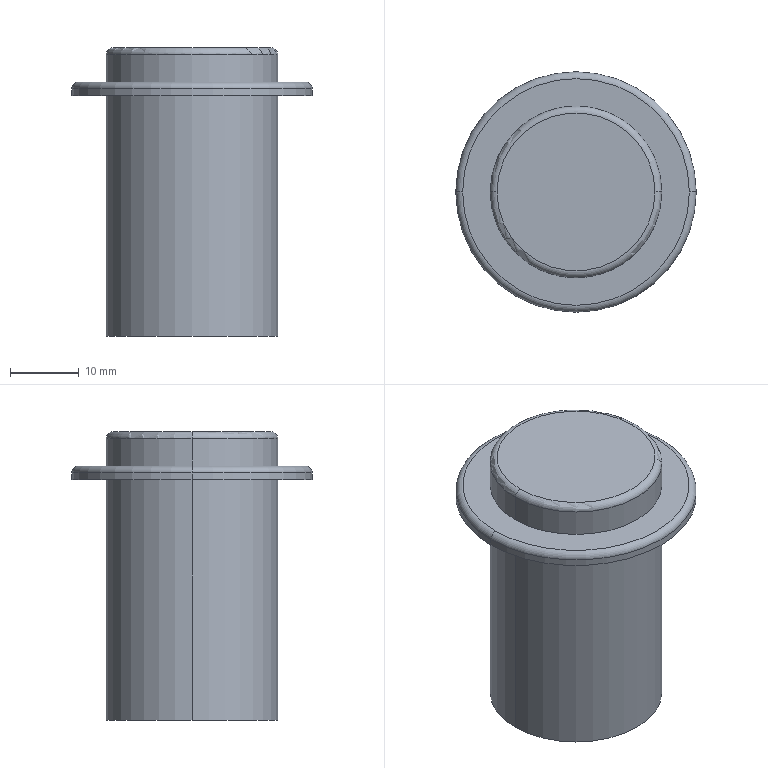Part | SolidWorks | features ICE 2, Extrusion 1, Fillet 1 | 1 solid | 14 faces | box 35 x 35 x 42 mm | volume 21519 mm3 | cylinder 6 | torus 4 | plane 4 | commonest cylinder face diameters 25 x4 35 x2
STEP:
#1=CARTESIAN_POINT('',(318.611,94.217,1.));
#2=VERTEX_POINT('',#1);
#3=CARTESIAN_POINT('',(353.611,94.217,1.));
#4=VERTEX_POINT('',#3);
#5=CARTESIAN_POINT('',(336.111,94.217,1.));
#6=DIRECTION('',(0.,0.,-1.));
#7=DIRECTION('',(1.,0.,0.));
#8=AXIS2_PLACEMENT_3D('',#5,#6,#7);
#9=CIRCLE('',#8,17.5);
#10=EDGE_CURVE('',#2,#4,#9,.T.);
#11=ORIENTED_EDGE('',*,*,#10,.F.);
#12=CARTESIAN_POINT('',(319.611,94.217,2.));
#13=VERTEX_POINT('',#12);
#14=CARTESIAN_POINT('',(319.611,94.217,1.));
#15=DIRECTION('',(0.,1.,0.));
#16=DIRECTION('',(-1.,0.,0.));
#17=AXIS2_PLACEMENT_3D('',#14,#15,#16);
#18=CIRCLE('',#17,1.);
#19=EDGE_CURVE('',#2,#13,#18,.T.);
#20=ORIENTED_EDGE('',*,*,#19,.T.);
#21=CARTESIAN_POINT('',(352.611,94.217,2.));
#22=VERTEX_POINT('',#21);
#23=CARTESIAN_POINT('',(336.111,94.217,2.));
#24=DIRECTION('',(0.,0.,1.));
#25=DIRECTION('',(1.,0.,0.));
#26=AXIS2_PLACEMENT_3D('',#23,#24,#25);
#27=CIRCLE('',#26,16.5);
#28=EDGE_CURVE('',#22,#13,#27,.T.);
#29=ORIENTED_EDGE('',*,*,#28,.F.);
#30=CARTESIAN_POINT('',(352.611,94.217,1.));
#31=DIRECTION('',(0.,-1.,0.));
#32=DIRECTION('',(1.,0.,0.));
#33=AXIS2_PLACEMENT_3D('',#30,#31,#32);
#34=CIRCLE('',#33,1.);
#35=EDGE_CURVE('',#4,#22,#34,.T.);
#36=ORIENTED_EDGE('',*,*,#35,.F.);
#37=EDGE_LOOP('',(#11,#20,#29,#36));
#38=FACE_OUTER_BOUND('',#37,.T.);
#39=CARTESIAN_POINT('',(336.111,94.217,1.));
#40=DIRECTION('',(0.,0.,1.));
#41=DIRECTION('',(1.,0.,0.));
#42=AXIS2_PLACEMENT_3D('',#39,#40,#41);
#43=TOROIDAL_SURFACE('',#42,16.5,1.);
#44=ADVANCED_FACE('',(#38),#43,.T.);
#45=CARTESIAN_POINT('',(323.611,94.217,6.));
#46=VERTEX_POINT('',#45);
#47=CARTESIAN_POINT('',(348.611,94.217,6.));
#48=VERTEX_POINT('',#47);
#49=CARTESIAN_POINT('',(336.111,94.217,6.));
#50=DIRECTION('',(0.,0.,-1.));
#51=DIRECTION('',(1.,0.,0.));
#52=AXIS2_PLACEMENT_3D('',#49,#50,#51);
#53=CIRCLE('',#52,12.5);
#54=EDGE_CURVE('',#46,#48,#53,.T.);
#55=ORIENTED_EDGE('',*,*,#54,.F.);
#56=CARTESIAN_POINT('',(324.611,94.217,7.));
#57=VERTEX_POINT('',#56);
#58=CARTESIAN_POINT('',(324.611,94.217,6.));
#59=DIRECTION('',(0.,1.,0.));
#60=DIRECTION('',(-1.,0.,0.));
#61=AXIS2_PLACEMENT_3D('',#58,#59,#60);
#62=CIRCLE('',#61,1.);
#63=EDGE_CURVE('',#46,#57,#62,.T.);
#64=ORIENTED_EDGE('',*,*,#63,.T.);
#65=CARTESIAN_POINT('',(347.611,94.217,7.));
#66=VERTEX_POINT('',#65);
#67=CARTESIAN_POINT('',(336.111,94.217,7.));
#68=DIRECTION('',(0.,0.,1.));
#69=DIRECTION('',(1.,0.,0.));
#70=AXIS2_PLACEMENT_3D('',#67,#68,#69);
#71=CIRCLE('',#70,11.5);
#72=EDGE_CURVE('',#66,#57,#71,.T.);
#73=ORIENTED_EDGE('',*,*,#72,.F.);
#74=CARTESIAN_POINT('',(347.611,94.217,6.));
#75=DIRECTION('',(0.,-1.,0.));
#76=DIRECTION('',(1.,0.,0.));
#77=AXIS2_PLACEMENT_3D('',#74,#75,#76);
#78=CIRCLE('',#77,1.);
#79=EDGE_CURVE('',#48,#66,#78,.T.);
#80=ORIENTED_EDGE('',*,*,#79,.F.);
#81=EDGE_LOOP('',(#55,#64,#73,#80));
#82=FACE_OUTER_BOUND('',#81,.T.);
#83=CARTESIAN_POINT('',(336.111,94.217,6.));
#84=DIRECTION('',(0.,0.,1.));
#85=DIRECTION('',(1.,0.,0.));
#86=AXIS2_PLACEMENT_3D('',#83,#84,#85);
#87=TOROIDAL_SURFACE('',#86,11.5,1.);
#88=ADVANCED_FACE('',(#82),#87,.T.);
#89=ORIENTED_EDGE('',*,*,#54,.T.);
#90=CARTESIAN_POINT('',(348.611,94.217,2.));
#91=VERTEX_POINT('',#90);
#92=CARTESIAN_POINT('',(348.611,94.217,7.));
#93=DIRECTION('',(0.,0.,-1.));
#94=VECTOR('',#93,1000.);
#95=LINE('',#92,#94);
#96=EDGE_CURVE('',#48,#91,#95,.T.);
#97=ORIENTED_EDGE('',*,*,#96,.T.);
#98=CARTESIAN_POINT('',(323.611,94.217,2.));
#99=VERTEX_POINT('',#98);
#100=CARTESIAN_POINT('',(336.111,94.217,2.));
#101=DIRECTION('',(0.,0.,1.));
#102=DIRECTION('',(1.,0.,0.));
#103=AXIS2_PLACEMENT_3D('',#100,#101,#102);
#104=CIRCLE('',#103,12.5);
#105=EDGE_CURVE('',#91,#99,#104,.T.);
#106=ORIENTED_EDGE('',*,*,#105,.T.);
#107=CARTESIAN_POINT('',(323.611,94.217,7.));
#108=DIRECTION('',(0.,0.,-1.));
#109=VECTOR('',#108,1000.);
#110=LINE('',#107,#109);
#111=EDGE_CURVE('',#46,#99,#110,.T.);
#112=ORIENTED_EDGE('',*,*,#111,.F.);
#113=EDGE_LOOP('',(#89,#97,#106,#112));
#114=FACE_OUTER_BOUND('',#113,.T.);
#115=CARTESIAN_POINT('',(336.111,94.217,7.));
#116=DIRECTION('',(0.,0.,-1.));
#117=DIRECTION('',(-1.,0.,0.));
#118=AXIS2_PLACEMENT_3D('',#115,#116,#117);
#119=CYLINDRICAL_SURFACE('',#118,12.5);
#120=ADVANCED_FACE('',(#114),#119,.T.);
#121=ORIENTED_EDGE('',*,*,#10,.T.);
#122=CARTESIAN_POINT('',(353.611,94.217,0.));
#123=VERTEX_POINT('',#122);
#124=CARTESIAN_POINT('',(353.611,94.217,2.));
#125=DIRECTION('',(0.,0.,-1.));
#126=VECTOR('',#125,1000.);
#127=LINE('',#124,#126);
#128=EDGE_CURVE('',#4,#123,#127,.T.);
#129=ORIENTED_EDGE('',*,*,#128,.T.);
#130=CARTESIAN_POINT('',(318.611,94.217,0.));
#131=VERTEX_POINT('',#130);
#132=CARTESIAN_POINT('',(336.111,94.217,0.));
#133=DIRECTION('',(0.,0.,1.));
#134=DIRECTION('',(1.,0.,0.));
#135=AXIS2_PLACEMENT_3D('',#132,#133,#134);
#136=CIRCLE('',#135,17.5);
#137=EDGE_CURVE('',#123,#131,#136,.T.);
#138=ORIENTED_EDGE('',*,*,#137,.T.);
#139=CARTESIAN_POINT('',(318.611,94.217,2.));
#140=DIRECTION('',(0.,0.,-1.));
#141=VECTOR('',#140,1000.);
#142=LINE('',#139,#141);
#143=EDGE_CURVE('',#2,#131,#142,.T.);
#144=ORIENTED_EDGE('',*,*,#143,.F.);
#145=EDGE_LOOP('',(#121,#129,#138,#144));
#146=FACE_OUTER_BOUND('',#145,.T.);
#147=CARTESIAN_POINT('',(336.111,94.217,2.));
#148=DIRECTION('',(0.,0.,-1.));
#149=DIRECTION('',(-1.,0.,0.));
#150=AXIS2_PLACEMENT_3D('',#147,#148,#149);
#151=CYLINDRICAL_SURFACE('',#150,17.5);
#152=ADVANCED_FACE('',(#146),#151,.T.);
#153=CARTESIAN_POINT('',(348.611,94.217,-35.));
#154=VERTEX_POINT('',#153);
#155=CARTESIAN_POINT('',(323.611,94.217,-35.));
#156=VERTEX_POINT('',#155);
#157=CARTESIAN_POINT('',(336.111,94.217,-35.));
#158=DIRECTION('',(0.,0.,1.));
#159=DIRECTION('',(1.,0.,0.));
#160=AXIS2_PLACEMENT_3D('',#157,#158,#159);
#161=CIRCLE('',#160,12.5);
#162=EDGE_CURVE('',#154,#156,#161,.T.);
#163=ORIENTED_EDGE('',*,*,#162,.T.);
#164=CARTESIAN_POINT('',(323.611,94.217,0.));
#165=VERTEX_POINT('',#164);
#166=CARTESIAN_POINT('',(323.611,94.217,-35.));
#167=DIRECTION('',(0.,0.,1.));
#168=VECTOR('',#167,1000.);
#169=LINE('',#166,#168);
#170=EDGE_CURVE('',#156,#165,#169,.T.);
#171=ORIENTED_EDGE('',*,*,#170,.T.);
#172=CARTESIAN_POINT('',(348.611,94.217,0.));
#173=VERTEX_POINT('',#172);
#174=CARTESIAN_POINT('',(336.111,94.217,0.));
#175=DIRECTION('',(0.,0.,1.));
#176=DIRECTION('',(1.,0.,0.));
#177=AXIS2_PLACEMENT_3D('',#174,#175,#176);
#178=CIRCLE('',#177,12.5);
#179=EDGE_CURVE('',#173,#165,#178,.T.);
#180=ORIENTED_EDGE('',*,*,#179,.F.);
#181=CARTESIAN_POINT('',(348.611,94.217,-35.));
#182=DIRECTION('',(0.,0.,1.));
#183=VECTOR('',#182,1000.);
#184=LINE('',#181,#183);
#185=EDGE_CURVE('',#154,#173,#184,.T.);
#186=ORIENTED_EDGE('',*,*,#185,.F.);
#187=EDGE_LOOP('',(#163,#171,#180,#186));
#188=FACE_OUTER_BOUND('',#187,.T.);
#189=CARTESIAN_POINT('',(336.111,94.217,-35.));
#190=DIRECTION('',(0.,0.,1.));
#191=DIRECTION('',(1.,0.,0.));
#192=AXIS2_PLACEMENT_3D('',#189,#190,#191);
#193=CYLINDRICAL_SURFACE('',#192,12.5);
#194=ADVANCED_FACE('',(#188),#193,.T.);
#195=ORIENTED_EDGE('',*,*,#170,.F.);
#196=CARTESIAN_POINT('',(336.111,94.217,-35.));
#197=DIRECTION('',(0.,0.,1.));
#198=DIRECTION('',(1.,0.,0.));
#199=AXIS2_PLACEMENT_3D('',#196,#197,#198);
#200=CIRCLE('',#199,12.5);
#201=EDGE_CURVE('',#156,#154,#200,.T.);
#202=ORIENTED_EDGE('',*,*,#201,.T.);
#203=ORIENTED_EDGE('',*,*,#185,.T.);
#204=CARTESIAN_POINT('',(336.111,94.217,0.));
#205=DIRECTION('',(0.,0.,1.));
#206=DIRECTION('',(1.,0.,0.));
#207=AXIS2_PLACEMENT_3D('',#204,#205,#206);
#208=CIRCLE('',#207,12.5);
#209=EDGE_CURVE('',#165,#173,#208,.T.);
#210=ORIENTED_EDGE('',*,*,#209,.F.);
#211=EDGE_LOOP('',(#195,#202,#203,#210));
#212=FACE_OUTER_BOUND('',#211,.T.);
#213=CARTESIAN_POINT('',(336.111,94.217,-35.));
#214=DIRECTION('',(0.,0.,1.));
#215=DIRECTION('',(1.,0.,0.));
#216=AXIS2_PLACEMENT_3D('',#213,#214,#215);
#217=CYLINDRICAL_SURFACE('',#216,12.5);
#218=ADVANCED_FACE('',(#212),#217,.T.);
#219=ORIENTED_EDGE('',*,*,#162,.F.);
#220=ORIENTED_EDGE('',*,*,#201,.F.);
#221=EDGE_LOOP('',(#219,#220));
#222=FACE_OUTER_BOUND('',#221,.T.);
#223=CARTESIAN_POINT('',(336.111,94.217,-35.));
#224=DIRECTION('',(0.,0.,1.));
#225=DIRECTION('',(1.,0.,0.));
#226=AXIS2_PLACEMENT_3D('',#223,#224,#225);
#227=PLANE('',#226);
#228=ADVANCED_FACE('',(#222),#227,.F.);
#229=ORIENTED_EDGE('',*,*,#128,.F.);
#230=CARTESIAN_POINT('',(336.111,94.217,1.));
#231=DIRECTION('',(0.,0.,-1.));
#232=DIRECTION('',(1.,0.,0.));
#233=AXIS2_PLACEMENT_3D('',#230,#231,#232);
#234=CIRCLE('',#233,17.5);
#235=EDGE_CURVE('',#4,#2,#234,.T.);
#236=ORIENTED_EDGE('',*,*,#235,.T.);
#237=ORIENTED_EDGE('',*,*,#143,.T.);
#238=CARTESIAN_POINT('',(336.111,94.217,0.));
#239=DIRECTION('',(0.,0.,1.));
#240=DIRECTION('',(1.,0.,0.));
#241=AXIS2_PLACEMENT_3D('',#238,#239,#240);
#242=CIRCLE('',#241,17.5);
#243=EDGE_CURVE('',#131,#123,#242,.T.);
#244=ORIENTED_EDGE('',*,*,#243,.T.);
#245=EDGE_LOOP('',(#229,#236,#237,#244));
#246=FACE_OUTER_BOUND('',#245,.T.);
#247=CARTESIAN_POINT('',(336.111,94.217,2.));
#248=DIRECTION('',(0.,0.,-1.));
#249=DIRECTION('',(-1.,0.,0.));
#250=AXIS2_PLACEMENT_3D('',#247,#248,#249);
#251=CYLINDRICAL_SURFACE('',#250,17.5);
#252=ADVANCED_FACE('',(#246),#251,.T.);
#253=ORIENTED_EDGE('',*,*,#28,.T.);
#254=CARTESIAN_POINT('',(336.111,94.217,2.));
#255=DIRECTION('',(0.,0.,1.));
#256=DIRECTION('',(1.,0.,0.));
#257=AXIS2_PLACEMENT_3D('',#254,#255,#256);
#258=CIRCLE('',#257,16.5);
#259=EDGE_CURVE('',#13,#22,#258,.T.);
#260=ORIENTED_EDGE('',*,*,#259,.T.);
#261=EDGE_LOOP('',(#253,#260));
#262=FACE_OUTER_BOUND('',#261,.T.);
#263=CARTESIAN_POINT('',(336.111,94.217,2.));
#264=DIRECTION('',(0.,0.,1.));
#265=DIRECTION('',(1.,0.,0.));
#266=AXIS2_PLACEMENT_3D('',#263,#264,#265);
#267=CIRCLE('',#266,12.5);
#268=EDGE_CURVE('',#99,#91,#267,.T.);
#269=ORIENTED_EDGE('',*,*,#268,.F.);
#270=ORIENTED_EDGE('',*,*,#105,.F.);
#271=EDGE_LOOP('',(#269,#270));
#272=FACE_BOUND('',#271,.T.);
#273=CARTESIAN_POINT('',(336.111,94.217,2.));
#274=DIRECTION('',(0.,0.,1.));
#275=DIRECTION('',(1.,0.,0.));
#276=AXIS2_PLACEMENT_3D('',#273,#274,#275);
#277=PLANE('',#276);
#278=ADVANCED_FACE('',(#262,#272),#277,.T.);
#279=ORIENTED_EDGE('',*,*,#179,.T.);
#280=ORIENTED_EDGE('',*,*,#209,.T.);
#281=EDGE_LOOP('',(#279,#280));
#282=FACE_BOUND('',#281,.T.);
#283=ORIENTED_EDGE('',*,*,#243,.F.);
#284=ORIENTED_EDGE('',*,*,#137,.F.);
#285=EDGE_LOOP('',(#283,#284));
#286=FACE_OUTER_BOUND('',#285,.T.);
#287=CARTESIAN_POINT('',(336.111,94.217,0.));
#288=DIRECTION('',(0.,0.,1.));
#289=DIRECTION('',(1.,0.,0.));
#290=AXIS2_PLACEMENT_3D('',#287,#288,#289);
#291=PLANE('',#290);
#292=ADVANCED_FACE('',(#282,#286),#291,.F.);
#293=ORIENTED_EDGE('',*,*,#96,.F.);
#294=CARTESIAN_POINT('',(336.111,94.217,6.));
#295=DIRECTION('',(0.,0.,-1.));
#296=DIRECTION('',(1.,0.,0.));
#297=AXIS2_PLACEMENT_3D('',#294,#295,#296);
#298=CIRCLE('',#297,12.5);
#299=EDGE_CURVE('',#48,#46,#298,.T.);
#300=ORIENTED_EDGE('',*,*,#299,.T.);
#301=ORIENTED_EDGE('',*,*,#111,.T.);
#302=ORIENTED_EDGE('',*,*,#268,.T.);
#303=EDGE_LOOP('',(#293,#300,#301,#302));
#304=FACE_OUTER_BOUND('',#303,.T.);
#305=CARTESIAN_POINT('',(336.111,94.217,7.));
#306=DIRECTION('',(0.,0.,-1.));
#307=DIRECTION('',(-1.,0.,0.));
#308=AXIS2_PLACEMENT_3D('',#305,#306,#307);
#309=CYLINDRICAL_SURFACE('',#308,12.5);
#310=ADVANCED_FACE('',(#304),#309,.T.);
#311=ORIENTED_EDGE('',*,*,#72,.T.);
#312=CARTESIAN_POINT('',(336.111,94.217,7.));
#313=DIRECTION('',(0.,0.,1.));
#314=DIRECTION('',(1.,0.,0.));
#315=AXIS2_PLACEMENT_3D('',#312,#313,#314);
#316=CIRCLE('',#315,11.5);
#317=EDGE_CURVE('',#57,#66,#316,.T.);
#318=ORIENTED_EDGE('',*,*,#317,.T.);
#319=EDGE_LOOP('',(#311,#318));
#320=FACE_OUTER_BOUND('',#319,.T.);
#321=CARTESIAN_POINT('',(336.111,94.217,7.));
#322=DIRECTION('',(0.,0.,1.));
#323=DIRECTION('',(1.,0.,0.));
#324=AXIS2_PLACEMENT_3D('',#321,#322,#323);
#325=PLANE('',#324);
#326=ADVANCED_FACE('',(#320),#325,.T.);
#327=ORIENTED_EDGE('',*,*,#63,.F.);
#328=ORIENTED_EDGE('',*,*,#299,.F.);
#329=ORIENTED_EDGE('',*,*,#79,.T.);
#330=ORIENTED_EDGE('',*,*,#317,.F.);
#331=EDGE_LOOP('',(#327,#328,#329,#330));
#332=FACE_OUTER_BOUND('',#331,.T.);
#333=CARTESIAN_POINT('',(336.111,94.217,6.));
#334=DIRECTION('',(0.,0.,1.));
#335=DIRECTION('',(1.,0.,0.));
#336=AXIS2_PLACEMENT_3D('',#333,#334,#335);
#337=TOROIDAL_SURFACE('',#336,11.5,1.);
#338=ADVANCED_FACE('',(#332),#337,.T.);
#339=ORIENTED_EDGE('',*,*,#19,.F.);
#340=ORIENTED_EDGE('',*,*,#235,.F.);
#341=ORIENTED_EDGE('',*,*,#35,.T.);
#342=ORIENTED_EDGE('',*,*,#259,.F.);
#343=EDGE_LOOP('',(#339,#340,#341,#342));
#344=FACE_OUTER_BOUND('',#343,.T.);
#345=CARTESIAN_POINT('',(336.111,94.217,1.));
#346=DIRECTION('',(0.,0.,1.));
#347=DIRECTION('',(1.,0.,0.));
#348=AXIS2_PLACEMENT_3D('',#345,#346,#347);
#349=TOROIDAL_SURFACE('',#348,16.5,1.);
#350=ADVANCED_FACE('',(#344),#349,.T.);
#351=CLOSED_SHELL('',(#44,#88,#120,#152,#194,#218,#228,#252,#278,#292,#310,#326,#338,#350));
#352=MANIFOLD_SOLID_BREP('',#351);
#353=CARTESIAN_POINT('',(0.,0.,0.));
#354=DIRECTION('',(0.,0.,1.));
#355=DIRECTION('',(1.,0.,0.));
#356=AXIS2_PLACEMENT_3D('',#353,#354,#355);
#357=(LENGTH_UNIT()NAMED_UNIT(*)SI_UNIT(.MILLI.,.METRE.));
#358=UNCERTAINTY_MEASURE_WITH_UNIT(LENGTH_MEASURE(0.00001),#357,'','');
#359=(NAMED_UNIT(*)PLANE_ANGLE_UNIT()SI_UNIT($,.RADIAN.));
#360=(NAMED_UNIT(*)SI_UNIT($,.STERADIAN.)SOLID_ANGLE_UNIT());
#361=(GEOMETRIC_REPRESENTATION_CONTEXT(3)GLOBAL_UNCERTAINTY_ASSIGNED_CONTEXT((#358))GLOBAL_UNIT_ASSIGNED_CONTEXT((#357,#359,#360))REPRESENTATION_CONTEXT('',''));
#362=ADVANCED_BREP_SHAPE_REPRESENTATION('',(#352,#356),#361);